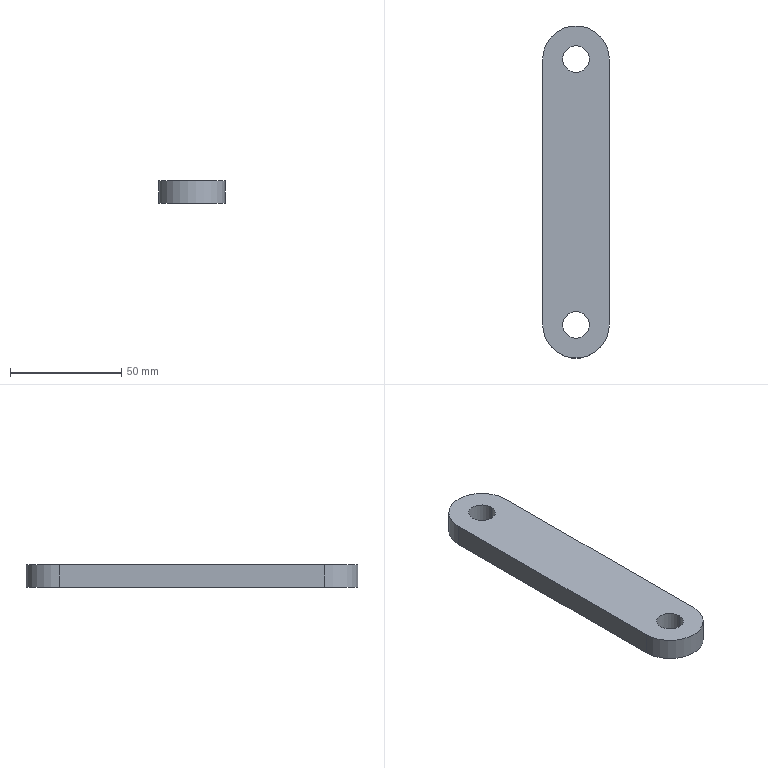Part | SolidWorks | features Extrusion 1 | 1 solid | 10 faces | box 30 x 149.604 x 10 mm | volume 40688 mm3 | cylinder 6 | plane 4 | commonest cylinder face diameters 12 x4 30 x2
STEP:
#1=CARTESIAN_POINT('',(79.,40.,0.));
#2=VERTEX_POINT('',#1);
#3=CARTESIAN_POINT('',(91.,40.,0.));
#4=VERTEX_POINT('',#3);
#5=CARTESIAN_POINT('',(85.,40.,0.));
#6=DIRECTION('',(0.,0.,1.));
#7=DIRECTION('',(1.,0.,0.));
#8=AXIS2_PLACEMENT_3D('',#5,#6,#7);
#9=CIRCLE('',#8,6.);
#10=EDGE_CURVE('',#2,#4,#9,.T.);
#11=ORIENTED_EDGE('',*,*,#10,.T.);
#12=CARTESIAN_POINT('',(91.,40.,-10.));
#13=VERTEX_POINT('',#12);
#14=CARTESIAN_POINT('',(91.,40.,0.));
#15=DIRECTION('',(0.,0.,-1.));
#16=VECTOR('',#15,1000.);
#17=LINE('',#14,#16);
#18=EDGE_CURVE('',#4,#13,#17,.T.);
#19=ORIENTED_EDGE('',*,*,#18,.T.);
#20=CARTESIAN_POINT('',(79.,40.,-10.));
#21=VERTEX_POINT('',#20);
#22=CARTESIAN_POINT('',(85.,40.,-10.));
#23=DIRECTION('',(0.,0.,1.));
#24=DIRECTION('',(1.,0.,0.));
#25=AXIS2_PLACEMENT_3D('',#22,#23,#24);
#26=CIRCLE('',#25,6.);
#27=EDGE_CURVE('',#21,#13,#26,.T.);
#28=ORIENTED_EDGE('',*,*,#27,.F.);
#29=CARTESIAN_POINT('',(79.,40.,0.));
#30=DIRECTION('',(0.,0.,-1.));
#31=VECTOR('',#30,1000.);
#32=LINE('',#29,#31);
#33=EDGE_CURVE('',#2,#21,#32,.T.);
#34=ORIENTED_EDGE('',*,*,#33,.F.);
#35=EDGE_LOOP('',(#11,#19,#28,#34));
#36=FACE_OUTER_BOUND('',#35,.T.);
#37=CARTESIAN_POINT('',(85.,40.,0.));
#38=DIRECTION('',(0.,0.,-1.));
#39=DIRECTION('',(-1.,0.,0.));
#40=AXIS2_PLACEMENT_3D('',#37,#38,#39);
#41=CYLINDRICAL_SURFACE('',#40,6.);
#42=ADVANCED_FACE('',(#36),#41,.F.);
#43=CARTESIAN_POINT('',(79.,-79.604,0.));
#44=VERTEX_POINT('',#43);
#45=CARTESIAN_POINT('',(91.,-79.604,0.));
#46=VERTEX_POINT('',#45);
#47=CARTESIAN_POINT('',(85.,-79.604,0.));
#48=DIRECTION('',(0.,0.,1.));
#49=DIRECTION('',(1.,0.,0.));
#50=AXIS2_PLACEMENT_3D('',#47,#48,#49);
#51=CIRCLE('',#50,6.);
#52=EDGE_CURVE('',#44,#46,#51,.T.);
#53=ORIENTED_EDGE('',*,*,#52,.T.);
#54=CARTESIAN_POINT('',(91.,-79.604,-10.));
#55=VERTEX_POINT('',#54);
#56=CARTESIAN_POINT('',(91.,-79.604,0.));
#57=DIRECTION('',(0.,0.,-1.));
#58=VECTOR('',#57,1000.);
#59=LINE('',#56,#58);
#60=EDGE_CURVE('',#46,#55,#59,.T.);
#61=ORIENTED_EDGE('',*,*,#60,.T.);
#62=CARTESIAN_POINT('',(79.,-79.604,-10.));
#63=VERTEX_POINT('',#62);
#64=CARTESIAN_POINT('',(85.,-79.604,-10.));
#65=DIRECTION('',(0.,0.,1.));
#66=DIRECTION('',(1.,0.,0.));
#67=AXIS2_PLACEMENT_3D('',#64,#65,#66);
#68=CIRCLE('',#67,6.);
#69=EDGE_CURVE('',#63,#55,#68,.T.);
#70=ORIENTED_EDGE('',*,*,#69,.F.);
#71=CARTESIAN_POINT('',(79.,-79.604,0.));
#72=DIRECTION('',(0.,0.,-1.));
#73=VECTOR('',#72,1000.);
#74=LINE('',#71,#73);
#75=EDGE_CURVE('',#44,#63,#74,.T.);
#76=ORIENTED_EDGE('',*,*,#75,.F.);
#77=EDGE_LOOP('',(#53,#61,#70,#76));
#78=FACE_OUTER_BOUND('',#77,.T.);
#79=CARTESIAN_POINT('',(85.,-79.604,0.));
#80=DIRECTION('',(0.,0.,-1.));
#81=DIRECTION('',(-1.,0.,0.));
#82=AXIS2_PLACEMENT_3D('',#79,#80,#81);
#83=CYLINDRICAL_SURFACE('',#82,6.);
#84=ADVANCED_FACE('',(#78),#83,.F.);
#85=ORIENTED_EDGE('',*,*,#52,.F.);
#86=CARTESIAN_POINT('',(85.,-79.604,0.));
#87=DIRECTION('',(0.,0.,1.));
#88=DIRECTION('',(1.,0.,0.));
#89=AXIS2_PLACEMENT_3D('',#86,#87,#88);
#90=CIRCLE('',#89,6.);
#91=EDGE_CURVE('',#46,#44,#90,.T.);
#92=ORIENTED_EDGE('',*,*,#91,.F.);
#93=EDGE_LOOP('',(#85,#92));
#94=FACE_BOUND('',#93,.T.);
#95=CARTESIAN_POINT('',(100.,40.,0.));
#96=VERTEX_POINT('',#95);
#97=CARTESIAN_POINT('',(70.,40.,0.));
#98=VERTEX_POINT('',#97);
#99=CARTESIAN_POINT('',(85.,40.,0.));
#100=DIRECTION('',(0.,0.,1.));
#101=DIRECTION('',(1.,0.,0.));
#102=AXIS2_PLACEMENT_3D('',#99,#100,#101);
#103=CIRCLE('',#102,15.);
#104=EDGE_CURVE('',#96,#98,#103,.T.);
#105=ORIENTED_EDGE('',*,*,#104,.T.);
#106=CARTESIAN_POINT('',(70.,-79.604,0.));
#107=VERTEX_POINT('',#106);
#108=CARTESIAN_POINT('',(70.,40.,0.));
#109=DIRECTION('',(0.,-1.,0.));
#110=VECTOR('',#109,1000.);
#111=LINE('',#108,#110);
#112=EDGE_CURVE('',#98,#107,#111,.T.);
#113=ORIENTED_EDGE('',*,*,#112,.T.);
#114=CARTESIAN_POINT('',(100.,-79.604,0.));
#115=VERTEX_POINT('',#114);
#116=CARTESIAN_POINT('',(85.,-79.604,0.));
#117=DIRECTION('',(0.,0.,1.));
#118=DIRECTION('',(1.,0.,0.));
#119=AXIS2_PLACEMENT_3D('',#116,#117,#118);
#120=CIRCLE('',#119,15.);
#121=EDGE_CURVE('',#107,#115,#120,.T.);
#122=ORIENTED_EDGE('',*,*,#121,.T.);
#123=CARTESIAN_POINT('',(100.,-79.604,0.));
#124=DIRECTION('',(0.,1.,0.));
#125=VECTOR('',#124,1000.);
#126=LINE('',#123,#125);
#127=EDGE_CURVE('',#115,#96,#126,.T.);
#128=ORIENTED_EDGE('',*,*,#127,.T.);
#129=EDGE_LOOP('',(#105,#113,#122,#128));
#130=FACE_OUTER_BOUND('',#129,.T.);
#131=ORIENTED_EDGE('',*,*,#10,.F.);
#132=CARTESIAN_POINT('',(85.,40.,0.));
#133=DIRECTION('',(0.,0.,1.));
#134=DIRECTION('',(1.,0.,0.));
#135=AXIS2_PLACEMENT_3D('',#132,#133,#134);
#136=CIRCLE('',#135,6.);
#137=EDGE_CURVE('',#4,#2,#136,.T.);
#138=ORIENTED_EDGE('',*,*,#137,.F.);
#139=EDGE_LOOP('',(#131,#138));
#140=FACE_BOUND('',#139,.T.);
#141=CARTESIAN_POINT('',(85.,40.,0.));
#142=DIRECTION('',(0.,0.,1.));
#143=DIRECTION('',(1.,0.,0.));
#144=AXIS2_PLACEMENT_3D('',#141,#142,#143);
#145=PLANE('',#144);
#146=ADVANCED_FACE('',(#94,#130,#140),#145,.T.);
#147=CARTESIAN_POINT('',(100.,40.,-10.));
#148=VERTEX_POINT('',#147);
#149=CARTESIAN_POINT('',(70.,40.,-10.));
#150=VERTEX_POINT('',#149);
#151=CARTESIAN_POINT('',(85.,40.,-10.));
#152=DIRECTION('',(0.,0.,1.));
#153=DIRECTION('',(1.,0.,0.));
#154=AXIS2_PLACEMENT_3D('',#151,#152,#153);
#155=CIRCLE('',#154,15.);
#156=EDGE_CURVE('',#148,#150,#155,.T.);
#157=ORIENTED_EDGE('',*,*,#156,.F.);
#158=CARTESIAN_POINT('',(100.,-79.604,-10.));
#159=VERTEX_POINT('',#158);
#160=CARTESIAN_POINT('',(100.,-79.604,-10.));
#161=DIRECTION('',(0.,1.,0.));
#162=VECTOR('',#161,1000.);
#163=LINE('',#160,#162);
#164=EDGE_CURVE('',#159,#148,#163,.T.);
#165=ORIENTED_EDGE('',*,*,#164,.F.);
#166=CARTESIAN_POINT('',(70.,-79.604,-10.));
#167=VERTEX_POINT('',#166);
#168=CARTESIAN_POINT('',(85.,-79.604,-10.));
#169=DIRECTION('',(0.,0.,1.));
#170=DIRECTION('',(1.,0.,0.));
#171=AXIS2_PLACEMENT_3D('',#168,#169,#170);
#172=CIRCLE('',#171,15.);
#173=EDGE_CURVE('',#167,#159,#172,.T.);
#174=ORIENTED_EDGE('',*,*,#173,.F.);
#175=CARTESIAN_POINT('',(70.,40.,-10.));
#176=DIRECTION('',(0.,-1.,0.));
#177=VECTOR('',#176,1000.);
#178=LINE('',#175,#177);
#179=EDGE_CURVE('',#150,#167,#178,.T.);
#180=ORIENTED_EDGE('',*,*,#179,.F.);
#181=EDGE_LOOP('',(#157,#165,#174,#180));
#182=FACE_OUTER_BOUND('',#181,.T.);
#183=ORIENTED_EDGE('',*,*,#69,.T.);
#184=CARTESIAN_POINT('',(85.,-79.604,-10.));
#185=DIRECTION('',(0.,0.,1.));
#186=DIRECTION('',(1.,0.,0.));
#187=AXIS2_PLACEMENT_3D('',#184,#185,#186);
#188=CIRCLE('',#187,6.);
#189=EDGE_CURVE('',#55,#63,#188,.T.);
#190=ORIENTED_EDGE('',*,*,#189,.T.);
#191=EDGE_LOOP('',(#183,#190));
#192=FACE_BOUND('',#191,.T.);
#193=ORIENTED_EDGE('',*,*,#27,.T.);
#194=CARTESIAN_POINT('',(85.,40.,-10.));
#195=DIRECTION('',(0.,0.,1.));
#196=DIRECTION('',(1.,0.,0.));
#197=AXIS2_PLACEMENT_3D('',#194,#195,#196);
#198=CIRCLE('',#197,6.);
#199=EDGE_CURVE('',#13,#21,#198,.T.);
#200=ORIENTED_EDGE('',*,*,#199,.T.);
#201=EDGE_LOOP('',(#193,#200));
#202=FACE_BOUND('',#201,.T.);
#203=CARTESIAN_POINT('',(85.,40.,-10.));
#204=DIRECTION('',(0.,0.,1.));
#205=DIRECTION('',(1.,0.,0.));
#206=AXIS2_PLACEMENT_3D('',#203,#204,#205);
#207=PLANE('',#206);
#208=ADVANCED_FACE('',(#182,#192,#202),#207,.F.);
#209=ORIENTED_EDGE('',*,*,#156,.T.);
#210=CARTESIAN_POINT('',(70.,40.,0.));
#211=DIRECTION('',(0.,0.,-1.));
#212=VECTOR('',#211,1000.);
#213=LINE('',#210,#212);
#214=EDGE_CURVE('',#98,#150,#213,.T.);
#215=ORIENTED_EDGE('',*,*,#214,.F.);
#216=ORIENTED_EDGE('',*,*,#104,.F.);
#217=CARTESIAN_POINT('',(100.,40.,0.));
#218=DIRECTION('',(0.,0.,-1.));
#219=VECTOR('',#218,1000.);
#220=LINE('',#217,#219);
#221=EDGE_CURVE('',#96,#148,#220,.T.);
#222=ORIENTED_EDGE('',*,*,#221,.T.);
#223=EDGE_LOOP('',(#209,#215,#216,#222));
#224=FACE_OUTER_BOUND('',#223,.T.);
#225=CARTESIAN_POINT('',(85.,40.,0.));
#226=DIRECTION('',(0.,0.,-1.));
#227=DIRECTION('',(-1.,0.,0.));
#228=AXIS2_PLACEMENT_3D('',#225,#226,#227);
#229=CYLINDRICAL_SURFACE('',#228,15.);
#230=ADVANCED_FACE('',(#224),#229,.T.);
#231=ORIENTED_EDGE('',*,*,#179,.T.);
#232=CARTESIAN_POINT('',(70.,-79.604,0.));
#233=DIRECTION('',(0.,0.,-1.));
#234=VECTOR('',#233,1000.);
#235=LINE('',#232,#234);
#236=EDGE_CURVE('',#107,#167,#235,.T.);
#237=ORIENTED_EDGE('',*,*,#236,.F.);
#238=ORIENTED_EDGE('',*,*,#112,.F.);
#239=ORIENTED_EDGE('',*,*,#214,.T.);
#240=EDGE_LOOP('',(#231,#237,#238,#239));
#241=FACE_OUTER_BOUND('',#240,.T.);
#242=CARTESIAN_POINT('',(70.,40.,0.));
#243=DIRECTION('',(1.,0.,0.));
#244=DIRECTION('',(0.,0.,-1.));
#245=AXIS2_PLACEMENT_3D('',#242,#243,#244);
#246=PLANE('',#245);
#247=ADVANCED_FACE('',(#241),#246,.F.);
#248=ORIENTED_EDGE('',*,*,#173,.T.);
#249=CARTESIAN_POINT('',(100.,-79.604,0.));
#250=DIRECTION('',(0.,0.,-1.));
#251=VECTOR('',#250,1000.);
#252=LINE('',#249,#251);
#253=EDGE_CURVE('',#115,#159,#252,.T.);
#254=ORIENTED_EDGE('',*,*,#253,.F.);
#255=ORIENTED_EDGE('',*,*,#121,.F.);
#256=ORIENTED_EDGE('',*,*,#236,.T.);
#257=EDGE_LOOP('',(#248,#254,#255,#256));
#258=FACE_OUTER_BOUND('',#257,.T.);
#259=CARTESIAN_POINT('',(85.,-79.604,0.));
#260=DIRECTION('',(0.,0.,-1.));
#261=DIRECTION('',(-1.,0.,0.));
#262=AXIS2_PLACEMENT_3D('',#259,#260,#261);
#263=CYLINDRICAL_SURFACE('',#262,15.);
#264=ADVANCED_FACE('',(#258),#263,.T.);
#265=ORIENTED_EDGE('',*,*,#164,.T.);
#266=ORIENTED_EDGE('',*,*,#221,.F.);
#267=ORIENTED_EDGE('',*,*,#127,.F.);
#268=ORIENTED_EDGE('',*,*,#253,.T.);
#269=EDGE_LOOP('',(#265,#266,#267,#268));
#270=FACE_OUTER_BOUND('',#269,.T.);
#271=CARTESIAN_POINT('',(100.,-79.604,0.));
#272=DIRECTION('',(-1.,0.,0.));
#273=DIRECTION('',(0.,0.,1.));
#274=AXIS2_PLACEMENT_3D('',#271,#272,#273);
#275=PLANE('',#274);
#276=ADVANCED_FACE('',(#270),#275,.F.);
#277=ORIENTED_EDGE('',*,*,#60,.F.);
#278=ORIENTED_EDGE('',*,*,#91,.T.);
#279=ORIENTED_EDGE('',*,*,#75,.T.);
#280=ORIENTED_EDGE('',*,*,#189,.F.);
#281=EDGE_LOOP('',(#277,#278,#279,#280));
#282=FACE_OUTER_BOUND('',#281,.T.);
#283=CARTESIAN_POINT('',(85.,-79.604,0.));
#284=DIRECTION('',(0.,0.,-1.));
#285=DIRECTION('',(-1.,0.,0.));
#286=AXIS2_PLACEMENT_3D('',#283,#284,#285);
#287=CYLINDRICAL_SURFACE('',#286,6.);
#288=ADVANCED_FACE('',(#282),#287,.F.);
#289=ORIENTED_EDGE('',*,*,#18,.F.);
#290=ORIENTED_EDGE('',*,*,#137,.T.);
#291=ORIENTED_EDGE('',*,*,#33,.T.);
#292=ORIENTED_EDGE('',*,*,#199,.F.);
#293=EDGE_LOOP('',(#289,#290,#291,#292));
#294=FACE_OUTER_BOUND('',#293,.T.);
#295=CARTESIAN_POINT('',(85.,40.,0.));
#296=DIRECTION('',(0.,0.,-1.));
#297=DIRECTION('',(-1.,0.,0.));
#298=AXIS2_PLACEMENT_3D('',#295,#296,#297);
#299=CYLINDRICAL_SURFACE('',#298,6.);
#300=ADVANCED_FACE('',(#294),#299,.F.);
#301=CLOSED_SHELL('',(#42,#84,#146,#208,#230,#247,#264,#276,#288,#300));
#302=MANIFOLD_SOLID_BREP('',#301);
#303=CARTESIAN_POINT('',(0.,0.,0.));
#304=DIRECTION('',(0.,0.,1.));
#305=DIRECTION('',(1.,0.,0.));
#306=AXIS2_PLACEMENT_3D('',#303,#304,#305);
#307=(LENGTH_UNIT()NAMED_UNIT(*)SI_UNIT(.MILLI.,.METRE.));
#308=UNCERTAINTY_MEASURE_WITH_UNIT(LENGTH_MEASURE(0.00001),#307,'','');
#309=(NAMED_UNIT(*)PLANE_ANGLE_UNIT()SI_UNIT($,.RADIAN.));
#310=(NAMED_UNIT(*)SI_UNIT($,.STERADIAN.)SOLID_ANGLE_UNIT());
#311=(GEOMETRIC_REPRESENTATION_CONTEXT(3)GLOBAL_UNCERTAINTY_ASSIGNED_CONTEXT((#308))GLOBAL_UNIT_ASSIGNED_CONTEXT((#307,#309,#310))REPRESENTATION_CONTEXT('',''));
#312=ADVANCED_BREP_SHAPE_REPRESENTATION('',(#302,#306),#311);